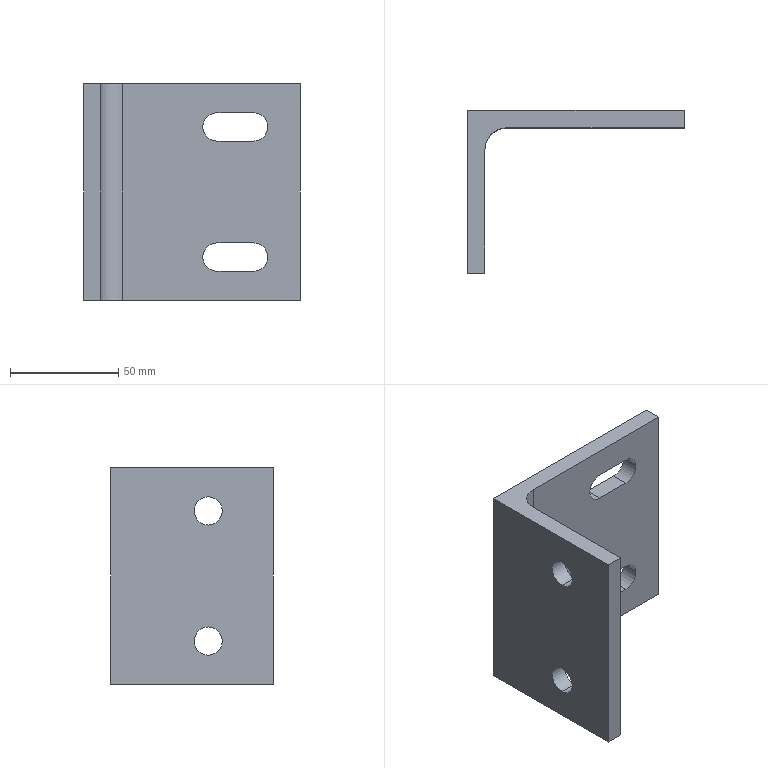Part | SolidWorks | features ICE 2, Extrusion 1, Fillet 1 | 1 solid | 21 faces | box 100 x 75 x 100 mm | volume 127963 mm3 | plane 12 | cylinder 9 | commonest cylinder face diameters 13 x8 20 x1
STEP:
#1=CARTESIAN_POINT('',(-100.,-45.,86.5));
#2=VERTEX_POINT('',#1);
#3=CARTESIAN_POINT('',(-100.,-45.,73.5));
#4=VERTEX_POINT('',#3);
#5=CARTESIAN_POINT('',(-100.,-45.,80.));
#6=DIRECTION('',(1.,0.,0.));
#7=DIRECTION('',(0.,1.,0.));
#8=AXIS2_PLACEMENT_3D('',#5,#6,#7);
#9=CIRCLE('',#8,6.5);
#10=EDGE_CURVE('',#2,#4,#9,.T.);
#11=ORIENTED_EDGE('',*,*,#10,.F.);
#12=CARTESIAN_POINT('',(-92.,-45.,86.5));
#13=VERTEX_POINT('',#12);
#14=CARTESIAN_POINT('',(-192.,-45.,86.5));
#15=DIRECTION('',(1.,0.,0.));
#16=VECTOR('',#15,1000.);
#17=LINE('',#14,#16);
#18=EDGE_CURVE('',#2,#13,#17,.T.);
#19=ORIENTED_EDGE('',*,*,#18,.T.);
#20=CARTESIAN_POINT('',(-92.,-45.,73.5));
#21=VERTEX_POINT('',#20);
#22=CARTESIAN_POINT('',(-92.,-45.,80.));
#23=DIRECTION('',(1.,0.,0.));
#24=DIRECTION('',(0.,0.,-1.));
#25=AXIS2_PLACEMENT_3D('',#22,#23,#24);
#26=CIRCLE('',#25,6.5);
#27=EDGE_CURVE('',#13,#21,#26,.T.);
#28=ORIENTED_EDGE('',*,*,#27,.T.);
#29=CARTESIAN_POINT('',(-192.,-45.,73.5));
#30=DIRECTION('',(1.,0.,0.));
#31=VECTOR('',#30,1000.);
#32=LINE('',#29,#31);
#33=EDGE_CURVE('',#4,#21,#32,.T.);
#34=ORIENTED_EDGE('',*,*,#33,.F.);
#35=EDGE_LOOP('',(#11,#19,#28,#34));
#36=FACE_OUTER_BOUND('',#35,.T.);
#37=CARTESIAN_POINT('',(-192.,-45.,80.));
#38=DIRECTION('',(1.,0.,0.));
#39=DIRECTION('',(0.,0.,-1.));
#40=AXIS2_PLACEMENT_3D('',#37,#38,#39);
#41=CYLINDRICAL_SURFACE('',#40,6.5);
#42=ADVANCED_FACE('',(#36),#41,.F.);
#43=CARTESIAN_POINT('',(-100.,-45.,26.5));
#44=VERTEX_POINT('',#43);
#45=CARTESIAN_POINT('',(-100.,-45.,13.5));
#46=VERTEX_POINT('',#45);
#47=CARTESIAN_POINT('',(-100.,-45.,20.));
#48=DIRECTION('',(1.,0.,0.));
#49=DIRECTION('',(0.,1.,0.));
#50=AXIS2_PLACEMENT_3D('',#47,#48,#49);
#51=CIRCLE('',#50,6.5);
#52=EDGE_CURVE('',#44,#46,#51,.T.);
#53=ORIENTED_EDGE('',*,*,#52,.F.);
#54=CARTESIAN_POINT('',(-92.,-45.,26.5));
#55=VERTEX_POINT('',#54);
#56=CARTESIAN_POINT('',(-192.,-45.,26.5));
#57=DIRECTION('',(1.,0.,0.));
#58=VECTOR('',#57,1000.);
#59=LINE('',#56,#58);
#60=EDGE_CURVE('',#44,#55,#59,.T.);
#61=ORIENTED_EDGE('',*,*,#60,.T.);
#62=CARTESIAN_POINT('',(-92.,-45.,13.5));
#63=VERTEX_POINT('',#62);
#64=CARTESIAN_POINT('',(-92.,-45.,20.));
#65=DIRECTION('',(1.,0.,0.));
#66=DIRECTION('',(0.,0.,-1.));
#67=AXIS2_PLACEMENT_3D('',#64,#65,#66);
#68=CIRCLE('',#67,6.5);
#69=EDGE_CURVE('',#55,#63,#68,.T.);
#70=ORIENTED_EDGE('',*,*,#69,.T.);
#71=CARTESIAN_POINT('',(-192.,-45.,13.5));
#72=DIRECTION('',(1.,0.,0.));
#73=VECTOR('',#72,1000.);
#74=LINE('',#71,#73);
#75=EDGE_CURVE('',#46,#63,#74,.T.);
#76=ORIENTED_EDGE('',*,*,#75,.F.);
#77=EDGE_LOOP('',(#53,#61,#70,#76));
#78=FACE_OUTER_BOUND('',#77,.T.);
#79=CARTESIAN_POINT('',(-192.,-45.,20.));
#80=DIRECTION('',(1.,0.,0.));
#81=DIRECTION('',(0.,0.,-1.));
#82=AXIS2_PLACEMENT_3D('',#79,#80,#81);
#83=CYLINDRICAL_SURFACE('',#82,6.5);
#84=ADVANCED_FACE('',(#78),#83,.F.);
#85=CARTESIAN_POINT('',(0.,-8.,0.));
#86=VERTEX_POINT('',#85);
#87=CARTESIAN_POINT('',(0.,0.,0.));
#88=VERTEX_POINT('',#87);
#89=CARTESIAN_POINT('',(0.,0.,0.));
#90=DIRECTION('',(0.,1.,0.));
#91=VECTOR('',#90,1000.);
#92=LINE('',#89,#91);
#93=EDGE_CURVE('',#86,#88,#92,.T.);
#94=ORIENTED_EDGE('',*,*,#93,.T.);
#95=CARTESIAN_POINT('',(0.,0.,100.));
#96=VERTEX_POINT('',#95);
#97=CARTESIAN_POINT('',(0.,0.,100.));
#98=DIRECTION('',(0.,0.,-1.));
#99=VECTOR('',#98,1000.);
#100=LINE('',#97,#99);
#101=EDGE_CURVE('',#96,#88,#100,.T.);
#102=ORIENTED_EDGE('',*,*,#101,.F.);
#103=CARTESIAN_POINT('',(0.,-8.,100.));
#104=VERTEX_POINT('',#103);
#105=CARTESIAN_POINT('',(0.,0.,100.));
#106=DIRECTION('',(0.,1.,0.));
#107=VECTOR('',#106,1000.);
#108=LINE('',#105,#107);
#109=EDGE_CURVE('',#104,#96,#108,.T.);
#110=ORIENTED_EDGE('',*,*,#109,.F.);
#111=CARTESIAN_POINT('',(0.,-8.,100.));
#112=DIRECTION('',(0.,0.,-1.));
#113=VECTOR('',#112,1000.);
#114=LINE('',#111,#113);
#115=EDGE_CURVE('',#104,#86,#114,.T.);
#116=ORIENTED_EDGE('',*,*,#115,.T.);
#117=EDGE_LOOP('',(#94,#102,#110,#116));
#118=FACE_OUTER_BOUND('',#117,.T.);
#119=CARTESIAN_POINT('',(0.,0.,100.));
#120=DIRECTION('',(-1.,0.,0.));
#121=DIRECTION('',(0.,0.,1.));
#122=AXIS2_PLACEMENT_3D('',#119,#120,#121);
#123=PLANE('',#122);
#124=ADVANCED_FACE('',(#118),#123,.F.);
#125=CARTESIAN_POINT('',(-38.5,0.,26.5));
#126=VERTEX_POINT('',#125);
#127=CARTESIAN_POINT('',(-21.5,0.,26.5));
#128=VERTEX_POINT('',#127);
#129=CARTESIAN_POINT('',(-38.5,0.,26.5));
#130=DIRECTION('',(1.,0.,0.));
#131=VECTOR('',#130,1000.);
#132=LINE('',#129,#131);
#133=EDGE_CURVE('',#126,#128,#132,.T.);
#134=ORIENTED_EDGE('',*,*,#133,.F.);
#135=CARTESIAN_POINT('',(-38.5,0.,13.5));
#136=VERTEX_POINT('',#135);
#137=CARTESIAN_POINT('',(-38.5,0.,20.));
#138=DIRECTION('',(0.,1.,0.));
#139=DIRECTION('',(0.,0.,1.));
#140=AXIS2_PLACEMENT_3D('',#137,#138,#139);
#141=CIRCLE('',#140,6.5);
#142=EDGE_CURVE('',#136,#126,#141,.T.);
#143=ORIENTED_EDGE('',*,*,#142,.F.);
#144=CARTESIAN_POINT('',(-21.5,0.,13.5));
#145=VERTEX_POINT('',#144);
#146=CARTESIAN_POINT('',(-38.5,0.,13.5));
#147=DIRECTION('',(-1.,0.,0.));
#148=VECTOR('',#147,1000.);
#149=LINE('',#146,#148);
#150=EDGE_CURVE('',#145,#136,#149,.T.);
#151=ORIENTED_EDGE('',*,*,#150,.F.);
#152=CARTESIAN_POINT('',(-21.5,0.,20.));
#153=DIRECTION('',(0.,1.,0.));
#154=DIRECTION('',(0.,0.,1.));
#155=AXIS2_PLACEMENT_3D('',#152,#153,#154);
#156=CIRCLE('',#155,6.5);
#157=EDGE_CURVE('',#128,#145,#156,.T.);
#158=ORIENTED_EDGE('',*,*,#157,.F.);
#159=EDGE_LOOP('',(#134,#143,#151,#158));
#160=FACE_BOUND('',#159,.T.);
#161=CARTESIAN_POINT('',(-38.5,0.,86.5));
#162=VERTEX_POINT('',#161);
#163=CARTESIAN_POINT('',(-21.5,0.,86.5));
#164=VERTEX_POINT('',#163);
#165=CARTESIAN_POINT('',(-38.5,0.,86.5));
#166=DIRECTION('',(1.,0.,0.));
#167=VECTOR('',#166,1000.);
#168=LINE('',#165,#167);
#169=EDGE_CURVE('',#162,#164,#168,.T.);
#170=ORIENTED_EDGE('',*,*,#169,.F.);
#171=CARTESIAN_POINT('',(-38.5,0.,73.5));
#172=VERTEX_POINT('',#171);
#173=CARTESIAN_POINT('',(-38.5,0.,80.));
#174=DIRECTION('',(0.,1.,0.));
#175=DIRECTION('',(0.,0.,1.));
#176=AXIS2_PLACEMENT_3D('',#173,#174,#175);
#177=CIRCLE('',#176,6.5);
#178=EDGE_CURVE('',#172,#162,#177,.T.);
#179=ORIENTED_EDGE('',*,*,#178,.F.);
#180=CARTESIAN_POINT('',(-21.5,0.,73.5));
#181=VERTEX_POINT('',#180);
#182=CARTESIAN_POINT('',(-38.5,0.,73.5));
#183=DIRECTION('',(-1.,0.,0.));
#184=VECTOR('',#183,1000.);
#185=LINE('',#182,#184);
#186=EDGE_CURVE('',#181,#172,#185,.T.);
#187=ORIENTED_EDGE('',*,*,#186,.F.);
#188=CARTESIAN_POINT('',(-21.5,0.,80.));
#189=DIRECTION('',(0.,1.,0.));
#190=DIRECTION('',(0.,0.,1.));
#191=AXIS2_PLACEMENT_3D('',#188,#189,#190);
#192=CIRCLE('',#191,6.5);
#193=EDGE_CURVE('',#164,#181,#192,.T.);
#194=ORIENTED_EDGE('',*,*,#193,.F.);
#195=EDGE_LOOP('',(#170,#179,#187,#194));
#196=FACE_BOUND('',#195,.T.);
#197=CARTESIAN_POINT('',(-100.,0.,0.));
#198=VERTEX_POINT('',#197);
#199=CARTESIAN_POINT('',(0.,0.,0.));
#200=DIRECTION('',(-1.,0.,0.));
#201=VECTOR('',#200,1000.);
#202=LINE('',#199,#201);
#203=EDGE_CURVE('',#88,#198,#202,.T.);
#204=ORIENTED_EDGE('',*,*,#203,.T.);
#205=CARTESIAN_POINT('',(-100.,0.,100.));
#206=VERTEX_POINT('',#205);
#207=CARTESIAN_POINT('',(-100.,0.,100.));
#208=DIRECTION('',(0.,0.,-1.));
#209=VECTOR('',#208,1000.);
#210=LINE('',#207,#209);
#211=EDGE_CURVE('',#206,#198,#210,.T.);
#212=ORIENTED_EDGE('',*,*,#211,.F.);
#213=CARTESIAN_POINT('',(0.,0.,100.));
#214=DIRECTION('',(-1.,0.,0.));
#215=VECTOR('',#214,1000.);
#216=LINE('',#213,#215);
#217=EDGE_CURVE('',#96,#206,#216,.T.);
#218=ORIENTED_EDGE('',*,*,#217,.F.);
#219=ORIENTED_EDGE('',*,*,#101,.T.);
#220=EDGE_LOOP('',(#204,#212,#218,#219));
#221=FACE_OUTER_BOUND('',#220,.T.);
#222=CARTESIAN_POINT('',(0.,0.,100.));
#223=DIRECTION('',(0.,-1.,0.));
#224=DIRECTION('',(0.,0.,-1.));
#225=AXIS2_PLACEMENT_3D('',#222,#223,#224);
#226=PLANE('',#225);
#227=ADVANCED_FACE('',(#160,#196,#221),#226,.F.);
#228=CARTESIAN_POINT('',(-100.,-45.,80.));
#229=DIRECTION('',(1.,0.,0.));
#230=DIRECTION('',(0.,1.,0.));
#231=AXIS2_PLACEMENT_3D('',#228,#229,#230);
#232=CIRCLE('',#231,6.5);
#233=EDGE_CURVE('',#4,#2,#232,.T.);
#234=ORIENTED_EDGE('',*,*,#233,.T.);
#235=ORIENTED_EDGE('',*,*,#10,.T.);
#236=EDGE_LOOP('',(#234,#235));
#237=FACE_BOUND('',#236,.T.);
#238=CARTESIAN_POINT('',(-100.,-45.,20.));
#239=DIRECTION('',(1.,0.,0.));
#240=DIRECTION('',(0.,1.,0.));
#241=AXIS2_PLACEMENT_3D('',#238,#239,#240);
#242=CIRCLE('',#241,6.5);
#243=EDGE_CURVE('',#46,#44,#242,.T.);
#244=ORIENTED_EDGE('',*,*,#243,.T.);
#245=ORIENTED_EDGE('',*,*,#52,.T.);
#246=EDGE_LOOP('',(#244,#245));
#247=FACE_BOUND('',#246,.T.);
#248=CARTESIAN_POINT('',(-100.,-75.,0.));
#249=VERTEX_POINT('',#248);
#250=CARTESIAN_POINT('',(-100.,0.,0.));
#251=DIRECTION('',(0.,-1.,0.));
#252=VECTOR('',#251,1000.);
#253=LINE('',#250,#252);
#254=EDGE_CURVE('',#198,#249,#253,.T.);
#255=ORIENTED_EDGE('',*,*,#254,.T.);
#256=CARTESIAN_POINT('',(-100.,-75.,100.));
#257=VERTEX_POINT('',#256);
#258=CARTESIAN_POINT('',(-100.,-75.,100.));
#259=DIRECTION('',(0.,0.,-1.));
#260=VECTOR('',#259,1000.);
#261=LINE('',#258,#260);
#262=EDGE_CURVE('',#257,#249,#261,.T.);
#263=ORIENTED_EDGE('',*,*,#262,.F.);
#264=CARTESIAN_POINT('',(-100.,0.,100.));
#265=DIRECTION('',(0.,-1.,0.));
#266=VECTOR('',#265,1000.);
#267=LINE('',#264,#266);
#268=EDGE_CURVE('',#206,#257,#267,.T.);
#269=ORIENTED_EDGE('',*,*,#268,.F.);
#270=ORIENTED_EDGE('',*,*,#211,.T.);
#271=EDGE_LOOP('',(#255,#263,#269,#270));
#272=FACE_OUTER_BOUND('',#271,.T.);
#273=CARTESIAN_POINT('',(-100.,0.,100.));
#274=DIRECTION('',(1.,0.,0.));
#275=DIRECTION('',(0.,1.,0.));
#276=AXIS2_PLACEMENT_3D('',#273,#274,#275);
#277=PLANE('',#276);
#278=ADVANCED_FACE('',(#237,#247,#272),#277,.F.);
#279=CARTESIAN_POINT('',(-92.,-75.,0.));
#280=VERTEX_POINT('',#279);
#281=CARTESIAN_POINT('',(-92.,-75.,0.));
#282=DIRECTION('',(1.,0.,0.));
#283=VECTOR('',#282,1000.);
#284=LINE('',#281,#283);
#285=EDGE_CURVE('',#249,#280,#284,.T.);
#286=ORIENTED_EDGE('',*,*,#285,.T.);
#287=CARTESIAN_POINT('',(-92.,-75.,100.));
#288=VERTEX_POINT('',#287);
#289=CARTESIAN_POINT('',(-92.,-75.,100.));
#290=DIRECTION('',(0.,0.,-1.));
#291=VECTOR('',#290,1000.);
#292=LINE('',#289,#291);
#293=EDGE_CURVE('',#288,#280,#292,.T.);
#294=ORIENTED_EDGE('',*,*,#293,.F.);
#295=CARTESIAN_POINT('',(-92.,-75.,100.));
#296=DIRECTION('',(1.,0.,0.));
#297=VECTOR('',#296,1000.);
#298=LINE('',#295,#297);
#299=EDGE_CURVE('',#257,#288,#298,.T.);
#300=ORIENTED_EDGE('',*,*,#299,.F.);
#301=ORIENTED_EDGE('',*,*,#262,.T.);
#302=EDGE_LOOP('',(#286,#294,#300,#301));
#303=FACE_OUTER_BOUND('',#302,.T.);
#304=CARTESIAN_POINT('',(-92.,-75.,100.));
#305=DIRECTION('',(0.,1.,0.));
#306=DIRECTION('',(0.,0.,1.));
#307=AXIS2_PLACEMENT_3D('',#304,#305,#306);
#308=PLANE('',#307);
#309=ADVANCED_FACE('',(#303),#308,.F.);
#310=CARTESIAN_POINT('',(-92.,-45.,80.));
#311=DIRECTION('',(1.,0.,0.));
#312=DIRECTION('',(0.,0.,-1.));
#313=AXIS2_PLACEMENT_3D('',#310,#311,#312);
#314=CIRCLE('',#313,6.5);
#315=EDGE_CURVE('',#21,#13,#314,.T.);
#316=ORIENTED_EDGE('',*,*,#315,.F.);
#317=ORIENTED_EDGE('',*,*,#27,.F.);
#318=EDGE_LOOP('',(#316,#317));
#319=FACE_BOUND('',#318,.T.);
#320=CARTESIAN_POINT('',(-92.,-45.,20.));
#321=DIRECTION('',(1.,0.,0.));
#322=DIRECTION('',(0.,0.,-1.));
#323=AXIS2_PLACEMENT_3D('',#320,#321,#322);
#324=CIRCLE('',#323,6.5);
#325=EDGE_CURVE('',#63,#55,#324,.T.);
#326=ORIENTED_EDGE('',*,*,#325,.F.);
#327=ORIENTED_EDGE('',*,*,#69,.F.);
#328=EDGE_LOOP('',(#326,#327));
#329=FACE_BOUND('',#328,.T.);
#330=CARTESIAN_POINT('',(-92.,-18.,0.));
#331=VERTEX_POINT('',#330);
#332=CARTESIAN_POINT('',(-92.,-8.,0.));
#333=DIRECTION('',(0.,1.,0.));
#334=VECTOR('',#333,1000.);
#335=LINE('',#332,#334);
#336=EDGE_CURVE('',#280,#331,#335,.T.);
#337=ORIENTED_EDGE('',*,*,#336,.T.);
#338=CARTESIAN_POINT('',(-92.,-18.,100.));
#339=VERTEX_POINT('',#338);
#340=CARTESIAN_POINT('',(-92.,-18.,100.));
#341=DIRECTION('',(0.,0.,1.));
#342=VECTOR('',#341,1000.);
#343=LINE('',#340,#342);
#344=EDGE_CURVE('',#331,#339,#343,.T.);
#345=ORIENTED_EDGE('',*,*,#344,.T.);
#346=CARTESIAN_POINT('',(-92.,-8.,100.));
#347=DIRECTION('',(0.,1.,0.));
#348=VECTOR('',#347,1000.);
#349=LINE('',#346,#348);
#350=EDGE_CURVE('',#288,#339,#349,.T.);
#351=ORIENTED_EDGE('',*,*,#350,.F.);
#352=ORIENTED_EDGE('',*,*,#293,.T.);
#353=EDGE_LOOP('',(#337,#345,#351,#352));
#354=FACE_OUTER_BOUND('',#353,.T.);
#355=CARTESIAN_POINT('',(-92.,-8.,100.));
#356=DIRECTION('',(-1.,0.,0.));
#357=DIRECTION('',(0.,0.,1.));
#358=AXIS2_PLACEMENT_3D('',#355,#356,#357);
#359=PLANE('',#358);
#360=ADVANCED_FACE('',(#319,#329,#354),#359,.F.);
#361=CARTESIAN_POINT('',(-21.5,-8.,13.5));
#362=VERTEX_POINT('',#361);
#363=CARTESIAN_POINT('',(-38.5,-8.,13.5));
#364=VERTEX_POINT('',#363);
#365=CARTESIAN_POINT('',(0.,-8.,13.5));
#366=DIRECTION('',(-1.,0.,0.));
#367=VECTOR('',#366,1000.);
#368=LINE('',#365,#367);
#369=EDGE_CURVE('',#362,#364,#368,.T.);
#370=ORIENTED_EDGE('',*,*,#369,.T.);
#371=CARTESIAN_POINT('',(-38.5,-8.,26.5));
#372=VERTEX_POINT('',#371);
#373=CARTESIAN_POINT('',(-38.5,-8.,20.));
#374=DIRECTION('',(0.,1.,0.));
#375=DIRECTION('',(0.,0.,1.));
#376=AXIS2_PLACEMENT_3D('',#373,#374,#375);
#377=CIRCLE('',#376,6.5);
#378=EDGE_CURVE('',#364,#372,#377,.T.);
#379=ORIENTED_EDGE('',*,*,#378,.T.);
#380=CARTESIAN_POINT('',(-21.5,-8.,26.5));
#381=VERTEX_POINT('',#380);
#382=CARTESIAN_POINT('',(0.,-8.,26.5));
#383=DIRECTION('',(1.,0.,0.));
#384=VECTOR('',#383,1000.);
#385=LINE('',#382,#384);
#386=EDGE_CURVE('',#372,#381,#385,.T.);
#387=ORIENTED_EDGE('',*,*,#386,.T.);
#388=CARTESIAN_POINT('',(-21.5,-8.,20.));
#389=DIRECTION('',(0.,1.,0.));
#390=DIRECTION('',(0.,0.,1.));
#391=AXIS2_PLACEMENT_3D('',#388,#389,#390);
#392=CIRCLE('',#391,6.5);
#393=EDGE_CURVE('',#381,#362,#392,.T.);
#394=ORIENTED_EDGE('',*,*,#393,.T.);
#395=EDGE_LOOP('',(#370,#379,#387,#394));
#396=FACE_BOUND('',#395,.T.);
#397=CARTESIAN_POINT('',(-21.5,-8.,73.5));
#398=VERTEX_POINT('',#397);
#399=CARTESIAN_POINT('',(-38.5,-8.,73.5));
#400=VERTEX_POINT('',#399);
#401=CARTESIAN_POINT('',(0.,-8.,73.5));
#402=DIRECTION('',(-1.,0.,0.));
#403=VECTOR('',#402,1000.);
#404=LINE('',#401,#403);
#405=EDGE_CURVE('',#398,#400,#404,.T.);
#406=ORIENTED_EDGE('',*,*,#405,.T.);
#407=CARTESIAN_POINT('',(-38.5,-8.,86.5));
#408=VERTEX_POINT('',#407);
#409=CARTESIAN_POINT('',(-38.5,-8.,80.));
#410=DIRECTION('',(0.,1.,0.));
#411=DIRECTION('',(0.,0.,1.));
#412=AXIS2_PLACEMENT_3D('',#409,#410,#411);
#413=CIRCLE('',#412,6.5);
#414=EDGE_CURVE('',#400,#408,#413,.T.);
#415=ORIENTED_EDGE('',*,*,#414,.T.);
#416=CARTESIAN_POINT('',(-21.5,-8.,86.5));
#417=VERTEX_POINT('',#416);
#418=CARTESIAN_POINT('',(0.,-8.,86.5));
#419=DIRECTION('',(1.,0.,0.));
#420=VECTOR('',#419,1000.);
#421=LINE('',#418,#420);
#422=EDGE_CURVE('',#408,#417,#421,.T.);
#423=ORIENTED_EDGE('',*,*,#422,.T.);
#424=CARTESIAN_POINT('',(-21.5,-8.,80.));
#425=DIRECTION('',(0.,1.,0.));
#426=DIRECTION('',(0.,0.,1.));
#427=AXIS2_PLACEMENT_3D('',#424,#425,#426);
#428=CIRCLE('',#427,6.5);
#429=EDGE_CURVE('',#417,#398,#428,.T.);
#430=ORIENTED_EDGE('',*,*,#429,.T.);
#431=EDGE_LOOP('',(#406,#415,#423,#430));
#432=FACE_BOUND('',#431,.T.);
#433=CARTESIAN_POINT('',(-82.,-8.,100.));
#434=VERTEX_POINT('',#433);
#435=CARTESIAN_POINT('',(0.,-8.,100.));
#436=DIRECTION('',(1.,0.,0.));
#437=VECTOR('',#436,1000.);
#438=LINE('',#435,#437);
#439=EDGE_CURVE('',#434,#104,#438,.T.);
#440=ORIENTED_EDGE('',*,*,#439,.F.);
#441=CARTESIAN_POINT('',(-82.,-8.,0.));
#442=VERTEX_POINT('',#441);
#443=CARTESIAN_POINT('',(-82.,-8.,0.));
#444=DIRECTION('',(0.,0.,-1.));
#445=VECTOR('',#444,1000.);
#446=LINE('',#443,#445);
#447=EDGE_CURVE('',#434,#442,#446,.T.);
#448=ORIENTED_EDGE('',*,*,#447,.T.);
#449=CARTESIAN_POINT('',(0.,-8.,0.));
#450=DIRECTION('',(1.,0.,0.));
#451=VECTOR('',#450,1000.);
#452=LINE('',#449,#451);
#453=EDGE_CURVE('',#442,#86,#452,.T.);
#454=ORIENTED_EDGE('',*,*,#453,.T.);
#455=ORIENTED_EDGE('',*,*,#115,.F.);
#456=EDGE_LOOP('',(#440,#448,#454,#455));
#457=FACE_OUTER_BOUND('',#456,.T.);
#458=CARTESIAN_POINT('',(0.,-8.,100.));
#459=DIRECTION('',(0.,1.,0.));
#460=DIRECTION('',(0.,0.,1.));
#461=AXIS2_PLACEMENT_3D('',#458,#459,#460);
#462=PLANE('',#461);
#463=ADVANCED_FACE('',(#396,#432,#457),#462,.F.);
#464=ORIENTED_EDGE('',*,*,#109,.T.);
#465=ORIENTED_EDGE('',*,*,#217,.T.);
#466=ORIENTED_EDGE('',*,*,#268,.T.);
#467=ORIENTED_EDGE('',*,*,#299,.T.);
#468=ORIENTED_EDGE('',*,*,#350,.T.);
#469=CARTESIAN_POINT('',(-82.,-18.,100.));
#470=DIRECTION('',(0.,0.,-1.));
#471=DIRECTION('',(-1.,0.,0.));
#472=AXIS2_PLACEMENT_3D('',#469,#470,#471);
#473=CIRCLE('',#472,10.);
#474=EDGE_CURVE('',#339,#434,#473,.T.);
#475=ORIENTED_EDGE('',*,*,#474,.T.);
#476=ORIENTED_EDGE('',*,*,#439,.T.);
#477=EDGE_LOOP('',(#464,#465,#466,#467,#468,#475,#476));
#478=FACE_OUTER_BOUND('',#477,.T.);
#479=CARTESIAN_POINT('',(0.,0.,100.));
#480=DIRECTION('',(0.,0.,-1.));
#481=DIRECTION('',(-1.,0.,0.));
#482=AXIS2_PLACEMENT_3D('',#479,#480,#481);
#483=PLANE('',#482);
#484=ADVANCED_FACE('',(#478),#483,.F.);
#485=ORIENTED_EDGE('',*,*,#93,.F.);
#486=ORIENTED_EDGE('',*,*,#453,.F.);
#487=CARTESIAN_POINT('',(-82.,-18.,0.));
#488=DIRECTION('',(0.,0.,1.));
#489=DIRECTION('',(-1.,0.,0.));
#490=AXIS2_PLACEMENT_3D('',#487,#488,#489);
#491=CIRCLE('',#490,10.);
#492=EDGE_CURVE('',#442,#331,#491,.T.);
#493=ORIENTED_EDGE('',*,*,#492,.T.);
#494=ORIENTED_EDGE('',*,*,#336,.F.);
#495=ORIENTED_EDGE('',*,*,#285,.F.);
#496=ORIENTED_EDGE('',*,*,#254,.F.);
#497=ORIENTED_EDGE('',*,*,#203,.F.);
#498=EDGE_LOOP('',(#485,#486,#493,#494,#495,#496,#497));
#499=FACE_OUTER_BOUND('',#498,.T.);
#500=CARTESIAN_POINT('',(0.,0.,0.));
#501=DIRECTION('',(0.,0.,-1.));
#502=DIRECTION('',(-1.,0.,0.));
#503=AXIS2_PLACEMENT_3D('',#500,#501,#502);
#504=PLANE('',#503);
#505=ADVANCED_FACE('',(#499),#504,.T.);
#506=CARTESIAN_POINT('',(-38.5,-100.,73.5));
#507=DIRECTION('',(0.,1.,0.));
#508=VECTOR('',#507,1000.);
#509=LINE('',#506,#508);
#510=EDGE_CURVE('',#400,#172,#509,.T.);
#511=ORIENTED_EDGE('',*,*,#510,.T.);
#512=ORIENTED_EDGE('',*,*,#178,.T.);
#513=CARTESIAN_POINT('',(-38.5,-100.,86.5));
#514=DIRECTION('',(0.,1.,0.));
#515=VECTOR('',#514,1000.);
#516=LINE('',#513,#515);
#517=EDGE_CURVE('',#408,#162,#516,.T.);
#518=ORIENTED_EDGE('',*,*,#517,.F.);
#519=ORIENTED_EDGE('',*,*,#414,.F.);
#520=EDGE_LOOP('',(#511,#512,#518,#519));
#521=FACE_OUTER_BOUND('',#520,.T.);
#522=CARTESIAN_POINT('',(-38.5,-100.,80.));
#523=DIRECTION('',(0.,1.,0.));
#524=DIRECTION('',(0.,0.,1.));
#525=AXIS2_PLACEMENT_3D('',#522,#523,#524);
#526=CYLINDRICAL_SURFACE('',#525,6.5);
#527=ADVANCED_FACE('',(#521),#526,.F.);
#528=CARTESIAN_POINT('',(-21.5,-100.,73.5));
#529=DIRECTION('',(0.,1.,0.));
#530=VECTOR('',#529,1000.);
#531=LINE('',#528,#530);
#532=EDGE_CURVE('',#398,#181,#531,.T.);
#533=ORIENTED_EDGE('',*,*,#532,.T.);
#534=ORIENTED_EDGE('',*,*,#186,.T.);
#535=ORIENTED_EDGE('',*,*,#510,.F.);
#536=ORIENTED_EDGE('',*,*,#405,.F.);
#537=EDGE_LOOP('',(#533,#534,#535,#536));
#538=FACE_OUTER_BOUND('',#537,.T.);
#539=CARTESIAN_POINT('',(-38.5,-100.,73.5));
#540=DIRECTION('',(0.,0.,-1.));
#541=DIRECTION('',(-1.,0.,0.));
#542=AXIS2_PLACEMENT_3D('',#539,#540,#541);
#543=PLANE('',#542);
#544=ADVANCED_FACE('',(#538),#543,.F.);
#545=CARTESIAN_POINT('',(-21.5,-100.,86.5));
#546=DIRECTION('',(0.,1.,0.));
#547=VECTOR('',#546,1000.);
#548=LINE('',#545,#547);
#549=EDGE_CURVE('',#417,#164,#548,.T.);
#550=ORIENTED_EDGE('',*,*,#549,.T.);
#551=ORIENTED_EDGE('',*,*,#193,.T.);
#552=ORIENTED_EDGE('',*,*,#532,.F.);
#553=ORIENTED_EDGE('',*,*,#429,.F.);
#554=EDGE_LOOP('',(#550,#551,#552,#553));
#555=FACE_OUTER_BOUND('',#554,.T.);
#556=CARTESIAN_POINT('',(-21.5,-100.,80.));
#557=DIRECTION('',(0.,1.,0.));
#558=DIRECTION('',(0.,0.,1.));
#559=AXIS2_PLACEMENT_3D('',#556,#557,#558);
#560=CYLINDRICAL_SURFACE('',#559,6.5);
#561=ADVANCED_FACE('',(#555),#560,.F.);
#562=ORIENTED_EDGE('',*,*,#517,.T.);
#563=ORIENTED_EDGE('',*,*,#169,.T.);
#564=ORIENTED_EDGE('',*,*,#549,.F.);
#565=ORIENTED_EDGE('',*,*,#422,.F.);
#566=EDGE_LOOP('',(#562,#563,#564,#565));
#567=FACE_OUTER_BOUND('',#566,.T.);
#568=CARTESIAN_POINT('',(-38.5,-100.,86.5));
#569=DIRECTION('',(0.,0.,1.));
#570=DIRECTION('',(1.,0.,0.));
#571=AXIS2_PLACEMENT_3D('',#568,#569,#570);
#572=PLANE('',#571);
#573=ADVANCED_FACE('',(#567),#572,.F.);
#574=CARTESIAN_POINT('',(-38.5,-100.,13.5));
#575=DIRECTION('',(0.,1.,0.));
#576=VECTOR('',#575,1000.);
#577=LINE('',#574,#576);
#578=EDGE_CURVE('',#364,#136,#577,.T.);
#579=ORIENTED_EDGE('',*,*,#578,.T.);
#580=ORIENTED_EDGE('',*,*,#142,.T.);
#581=CARTESIAN_POINT('',(-38.5,-100.,26.5));
#582=DIRECTION('',(0.,1.,0.));
#583=VECTOR('',#582,1000.);
#584=LINE('',#581,#583);
#585=EDGE_CURVE('',#372,#126,#584,.T.);
#586=ORIENTED_EDGE('',*,*,#585,.F.);
#587=ORIENTED_EDGE('',*,*,#378,.F.);
#588=EDGE_LOOP('',(#579,#580,#586,#587));
#589=FACE_OUTER_BOUND('',#588,.T.);
#590=CARTESIAN_POINT('',(-38.5,-100.,20.));
#591=DIRECTION('',(0.,1.,0.));
#592=DIRECTION('',(0.,0.,1.));
#593=AXIS2_PLACEMENT_3D('',#590,#591,#592);
#594=CYLINDRICAL_SURFACE('',#593,6.5);
#595=ADVANCED_FACE('',(#589),#594,.F.);
#596=CARTESIAN_POINT('',(-21.5,-100.,13.5));
#597=DIRECTION('',(0.,1.,0.));
#598=VECTOR('',#597,1000.);
#599=LINE('',#596,#598);
#600=EDGE_CURVE('',#362,#145,#599,.T.);
#601=ORIENTED_EDGE('',*,*,#600,.T.);
#602=ORIENTED_EDGE('',*,*,#150,.T.);
#603=ORIENTED_EDGE('',*,*,#578,.F.);
#604=ORIENTED_EDGE('',*,*,#369,.F.);
#605=EDGE_LOOP('',(#601,#602,#603,#604));
#606=FACE_OUTER_BOUND('',#605,.T.);
#607=CARTESIAN_POINT('',(-38.5,-100.,13.5));
#608=DIRECTION('',(0.,0.,-1.));
#609=DIRECTION('',(-1.,0.,0.));
#610=AXIS2_PLACEMENT_3D('',#607,#608,#609);
#611=PLANE('',#610);
#612=ADVANCED_FACE('',(#606),#611,.F.);
#613=CARTESIAN_POINT('',(-21.5,-100.,26.5));
#614=DIRECTION('',(0.,1.,0.));
#615=VECTOR('',#614,1000.);
#616=LINE('',#613,#615);
#617=EDGE_CURVE('',#381,#128,#616,.T.);
#618=ORIENTED_EDGE('',*,*,#617,.T.);
#619=ORIENTED_EDGE('',*,*,#157,.T.);
#620=ORIENTED_EDGE('',*,*,#600,.F.);
#621=ORIENTED_EDGE('',*,*,#393,.F.);
#622=EDGE_LOOP('',(#618,#619,#620,#621));
#623=FACE_OUTER_BOUND('',#622,.T.);
#624=CARTESIAN_POINT('',(-21.5,-100.,20.));
#625=DIRECTION('',(0.,1.,0.));
#626=DIRECTION('',(0.,0.,1.));
#627=AXIS2_PLACEMENT_3D('',#624,#625,#626);
#628=CYLINDRICAL_SURFACE('',#627,6.5);
#629=ADVANCED_FACE('',(#623),#628,.F.);
#630=ORIENTED_EDGE('',*,*,#585,.T.);
#631=ORIENTED_EDGE('',*,*,#133,.T.);
#632=ORIENTED_EDGE('',*,*,#617,.F.);
#633=ORIENTED_EDGE('',*,*,#386,.F.);
#634=EDGE_LOOP('',(#630,#631,#632,#633));
#635=FACE_OUTER_BOUND('',#634,.T.);
#636=CARTESIAN_POINT('',(-38.5,-100.,26.5));
#637=DIRECTION('',(0.,0.,1.));
#638=DIRECTION('',(1.,0.,0.));
#639=AXIS2_PLACEMENT_3D('',#636,#637,#638);
#640=PLANE('',#639);
#641=ADVANCED_FACE('',(#635),#640,.F.);
#642=ORIENTED_EDGE('',*,*,#60,.F.);
#643=ORIENTED_EDGE('',*,*,#243,.F.);
#644=ORIENTED_EDGE('',*,*,#75,.T.);
#645=ORIENTED_EDGE('',*,*,#325,.T.);
#646=EDGE_LOOP('',(#642,#643,#644,#645));
#647=FACE_OUTER_BOUND('',#646,.T.);
#648=CARTESIAN_POINT('',(-192.,-45.,20.));
#649=DIRECTION('',(1.,0.,0.));
#650=DIRECTION('',(0.,0.,-1.));
#651=AXIS2_PLACEMENT_3D('',#648,#649,#650);
#652=CYLINDRICAL_SURFACE('',#651,6.5);
#653=ADVANCED_FACE('',(#647),#652,.F.);
#654=ORIENTED_EDGE('',*,*,#18,.F.);
#655=ORIENTED_EDGE('',*,*,#233,.F.);
#656=ORIENTED_EDGE('',*,*,#33,.T.);
#657=ORIENTED_EDGE('',*,*,#315,.T.);
#658=EDGE_LOOP('',(#654,#655,#656,#657));
#659=FACE_OUTER_BOUND('',#658,.T.);
#660=CARTESIAN_POINT('',(-192.,-45.,80.));
#661=DIRECTION('',(1.,0.,0.));
#662=DIRECTION('',(0.,0.,-1.));
#663=AXIS2_PLACEMENT_3D('',#660,#661,#662);
#664=CYLINDRICAL_SURFACE('',#663,6.5);
#665=ADVANCED_FACE('',(#659),#664,.F.);
#666=ORIENTED_EDGE('',*,*,#474,.F.);
#667=ORIENTED_EDGE('',*,*,#344,.F.);
#668=ORIENTED_EDGE('',*,*,#492,.F.);
#669=ORIENTED_EDGE('',*,*,#447,.F.);
#670=EDGE_LOOP('',(#666,#667,#668,#669));
#671=FACE_OUTER_BOUND('',#670,.T.);
#672=CARTESIAN_POINT('',(-82.,-18.,100.));
#673=DIRECTION('',(0.,0.,1.));
#674=DIRECTION('',(1.,0.,0.));
#675=AXIS2_PLACEMENT_3D('',#672,#673,#674);
#676=CYLINDRICAL_SURFACE('',#675,10.);
#677=ADVANCED_FACE('',(#671),#676,.F.);
#678=CLOSED_SHELL('',(#42,#84,#124,#227,#278,#309,#360,#463,#484,#505,#527,#544,#561,#573,#595,#612,#629,#641,#653,#665,#677));
#679=MANIFOLD_SOLID_BREP('',#678);
#680=CARTESIAN_POINT('',(0.,0.,0.));
#681=DIRECTION('',(0.,0.,1.));
#682=DIRECTION('',(1.,0.,0.));
#683=AXIS2_PLACEMENT_3D('',#680,#681,#682);
#684=(LENGTH_UNIT()NAMED_UNIT(*)SI_UNIT(.MILLI.,.METRE.));
#685=UNCERTAINTY_MEASURE_WITH_UNIT(LENGTH_MEASURE(0.00001),#684,'','');
#686=(NAMED_UNIT(*)PLANE_ANGLE_UNIT()SI_UNIT($,.RADIAN.));
#687=(NAMED_UNIT(*)SI_UNIT($,.STERADIAN.)SOLID_ANGLE_UNIT());
#688=(GEOMETRIC_REPRESENTATION_CONTEXT(3)GLOBAL_UNCERTAINTY_ASSIGNED_CONTEXT((#685))GLOBAL_UNIT_ASSIGNED_CONTEXT((#684,#686,#687))REPRESENTATION_CONTEXT('',''));
#689=ADVANCED_BREP_SHAPE_REPRESENTATION('',(#679,#683),#688);